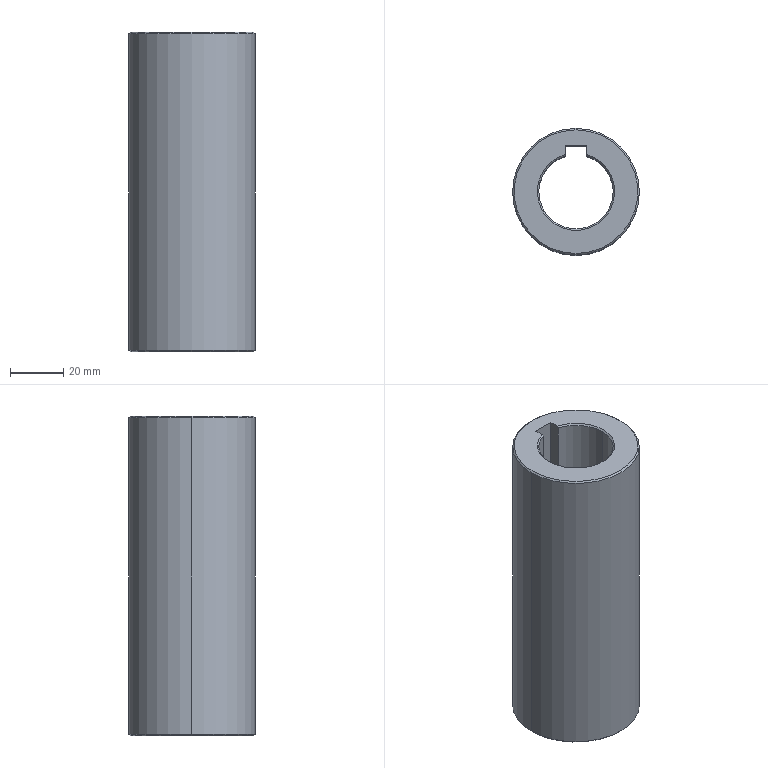Part | SolidWorks | features BaseBody 1 | 1 solid | 32 faces | box 47.6 x 47.6 x 120 mm | volume 130851 mm3 | cone 16 | cylinder 11 | plane 5 | commonest cylinder face diameters 28 x6 31.3 x3 47.6 x2
STEP:
#1=CARTESIAN_POINT('',(0.,23.8,-59.44));
#2=VERTEX_POINT('',#1);
#3=CARTESIAN_POINT('',(-23.8,0.,-59.44));
#4=VERTEX_POINT('',#3);
#5=CARTESIAN_POINT('',(0.,0.,-59.44));
#6=DIRECTION('',(0.,0.,1.));
#7=DIRECTION('',(1.,0.,0.));
#8=AXIS2_PLACEMENT_3D('',#5,#6,#7);
#9=CIRCLE('',#8,23.8);
#10=EDGE_CURVE('',#2,#4,#9,.T.);
#11=ORIENTED_EDGE('',*,*,#10,.T.);
#12=CARTESIAN_POINT('',(-23.8,0.,59.44));
#13=VERTEX_POINT('',#12);
#14=CARTESIAN_POINT('',(-23.8,0.,60.));
#15=DIRECTION('',(0.,0.,1.));
#16=VECTOR('',#15,1000.);
#17=LINE('',#14,#16);
#18=EDGE_CURVE('',#4,#13,#17,.T.);
#19=ORIENTED_EDGE('',*,*,#18,.T.);
#20=CARTESIAN_POINT('',(0.,23.8,59.44));
#21=VERTEX_POINT('',#20);
#22=CARTESIAN_POINT('',(0.,0.,59.44));
#23=DIRECTION('',(0.,0.,-1.));
#24=DIRECTION('',(1.,0.,0.));
#25=AXIS2_PLACEMENT_3D('',#22,#23,#24);
#26=CIRCLE('',#25,23.8);
#27=EDGE_CURVE('',#13,#21,#26,.T.);
#28=ORIENTED_EDGE('',*,*,#27,.T.);
#29=CARTESIAN_POINT('',(23.8,0.,59.44));
#30=VERTEX_POINT('',#29);
#31=CARTESIAN_POINT('',(0.,0.,59.44));
#32=DIRECTION('',(0.,0.,-1.));
#33=DIRECTION('',(1.,0.,0.));
#34=AXIS2_PLACEMENT_3D('',#31,#32,#33);
#35=CIRCLE('',#34,23.8);
#36=EDGE_CURVE('',#21,#30,#35,.T.);
#37=ORIENTED_EDGE('',*,*,#36,.T.);
#38=CARTESIAN_POINT('',(23.8,0.,-59.44));
#39=VERTEX_POINT('',#38);
#40=CARTESIAN_POINT('',(23.8,0.,60.));
#41=DIRECTION('',(0.,0.,1.));
#42=VECTOR('',#41,1000.);
#43=LINE('',#40,#42);
#44=EDGE_CURVE('',#39,#30,#43,.T.);
#45=ORIENTED_EDGE('',*,*,#44,.F.);
#46=CARTESIAN_POINT('',(0.,0.,-59.44));
#47=DIRECTION('',(0.,0.,1.));
#48=DIRECTION('',(1.,0.,0.));
#49=AXIS2_PLACEMENT_3D('',#46,#47,#48);
#50=CIRCLE('',#49,23.8);
#51=EDGE_CURVE('',#39,#2,#50,.T.);
#52=ORIENTED_EDGE('',*,*,#51,.T.);
#53=EDGE_LOOP('',(#11,#19,#28,#37,#45,#52));
#54=FACE_OUTER_BOUND('',#53,.T.);
#55=CARTESIAN_POINT('',(0.,0.,60.));
#56=DIRECTION('',(0.,0.,1.));
#57=DIRECTION('',(1.,0.,0.));
#58=AXIS2_PLACEMENT_3D('',#55,#56,#57);
#59=CYLINDRICAL_SURFACE('',#58,23.8);
#60=ADVANCED_FACE('',(#54),#59,.T.);
#61=CARTESIAN_POINT('',(0.,23.24,60.));
#62=VERTEX_POINT('',#61);
#63=CARTESIAN_POINT('',(0.,-23.24,60.));
#64=VERTEX_POINT('',#63);
#65=CARTESIAN_POINT('',(0.,0.,60.));
#66=DIRECTION('',(0.,0.,-1.));
#67=DIRECTION('',(0.,1.,0.));
#68=AXIS2_PLACEMENT_3D('',#65,#66,#67);
#69=CIRCLE('',#68,23.24);
#70=EDGE_CURVE('',#62,#64,#69,.T.);
#71=ORIENTED_EDGE('',*,*,#70,.T.);
#72=CARTESIAN_POINT('',(0.,-23.8,59.44));
#73=VERTEX_POINT('',#72);
#74=CARTESIAN_POINT('',(0.,-23.8,59.44));
#75=DIRECTION('',(0.,-0.7071,-0.7071));
#76=VECTOR('',#75,1000.);
#77=LINE('',#74,#76);
#78=EDGE_CURVE('',#64,#73,#77,.T.);
#79=ORIENTED_EDGE('',*,*,#78,.T.);
#80=CARTESIAN_POINT('',(0.,0.,59.44));
#81=DIRECTION('',(0.,0.,-1.));
#82=DIRECTION('',(1.,0.,0.));
#83=AXIS2_PLACEMENT_3D('',#80,#81,#82);
#84=CIRCLE('',#83,23.8);
#85=EDGE_CURVE('',#30,#73,#84,.T.);
#86=ORIENTED_EDGE('',*,*,#85,.F.);
#87=ORIENTED_EDGE('',*,*,#36,.F.);
#88=CARTESIAN_POINT('',(0.,23.8,59.44));
#89=DIRECTION('',(0.,0.7071,-0.7071));
#90=VECTOR('',#89,1000.);
#91=LINE('',#88,#90);
#92=EDGE_CURVE('',#62,#21,#91,.T.);
#93=ORIENTED_EDGE('',*,*,#92,.F.);
#94=EDGE_LOOP('',(#71,#79,#86,#87,#93));
#95=FACE_OUTER_BOUND('',#94,.T.);
#96=CARTESIAN_POINT('',(0.,0.,59.44));
#97=DIRECTION('',(0.,0.,-1.));
#98=DIRECTION('',(0.,1.,0.));
#99=AXIS2_PLACEMENT_3D('',#96,#97,#98);
#100=CONICAL_SURFACE('',#99,23.8,0.7854);
#101=ADVANCED_FACE('',(#95),#100,.T.);
#102=CARTESIAN_POINT('',(0.,-23.24,-60.));
#103=VERTEX_POINT('',#102);
#104=CARTESIAN_POINT('',(0.,23.24,-60.));
#105=VERTEX_POINT('',#104);
#106=CARTESIAN_POINT('',(0.,0.,-60.));
#107=DIRECTION('',(0.,0.,1.));
#108=DIRECTION('',(0.,-1.,0.));
#109=AXIS2_PLACEMENT_3D('',#106,#107,#108);
#110=CIRCLE('',#109,23.24);
#111=EDGE_CURVE('',#103,#105,#110,.T.);
#112=ORIENTED_EDGE('',*,*,#111,.T.);
#113=CARTESIAN_POINT('',(0.,23.8,-59.44));
#114=DIRECTION('',(0.,0.7071,0.7071));
#115=VECTOR('',#114,1000.);
#116=LINE('',#113,#115);
#117=EDGE_CURVE('',#105,#2,#116,.T.);
#118=ORIENTED_EDGE('',*,*,#117,.T.);
#119=ORIENTED_EDGE('',*,*,#51,.F.);
#120=CARTESIAN_POINT('',(0.,-23.8,-59.44));
#121=VERTEX_POINT('',#120);
#122=CARTESIAN_POINT('',(0.,0.,-59.44));
#123=DIRECTION('',(0.,0.,1.));
#124=DIRECTION('',(1.,0.,0.));
#125=AXIS2_PLACEMENT_3D('',#122,#123,#124);
#126=CIRCLE('',#125,23.8);
#127=EDGE_CURVE('',#121,#39,#126,.T.);
#128=ORIENTED_EDGE('',*,*,#127,.F.);
#129=CARTESIAN_POINT('',(0.,-23.8,-59.44));
#130=DIRECTION('',(0.,-0.7071,0.7071));
#131=VECTOR('',#130,1000.);
#132=LINE('',#129,#131);
#133=EDGE_CURVE('',#103,#121,#132,.T.);
#134=ORIENTED_EDGE('',*,*,#133,.F.);
#135=EDGE_LOOP('',(#112,#118,#119,#128,#134));
#136=FACE_OUTER_BOUND('',#135,.T.);
#137=CARTESIAN_POINT('',(0.,0.,-59.44));
#138=DIRECTION('',(0.,0.,1.));
#139=DIRECTION('',(0.,-1.,0.));
#140=AXIS2_PLACEMENT_3D('',#137,#138,#139);
#141=CONICAL_SURFACE('',#140,23.8,0.7854);
#142=ADVANCED_FACE('',(#136),#141,.T.);
#143=CARTESIAN_POINT('',(-14.,0.,59.44));
#144=VERTEX_POINT('',#143);
#145=CARTESIAN_POINT('',(14.,0.,59.44));
#146=VERTEX_POINT('',#145);
#147=CARTESIAN_POINT('',(0.,0.,59.44));
#148=DIRECTION('',(0.,0.,1.));
#149=DIRECTION('',(1.,0.,0.));
#150=AXIS2_PLACEMENT_3D('',#147,#148,#149);
#151=CIRCLE('',#150,14.);
#152=EDGE_CURVE('',#144,#146,#151,.T.);
#153=ORIENTED_EDGE('',*,*,#152,.F.);
#154=CARTESIAN_POINT('',(-14.56,0.,60.));
#155=VERTEX_POINT('',#154);
#156=CARTESIAN_POINT('',(-14.56,0.,60.));
#157=DIRECTION('',(-0.7071,0.,0.7071));
#158=VECTOR('',#157,1000.);
#159=LINE('',#156,#158);
#160=EDGE_CURVE('',#144,#155,#159,.T.);
#161=ORIENTED_EDGE('',*,*,#160,.T.);
#162=CARTESIAN_POINT('',(14.56,0.,60.));
#163=VERTEX_POINT('',#162);
#164=CARTESIAN_POINT('',(0.,0.,60.));
#165=DIRECTION('',(0.,0.,1.));
#166=DIRECTION('',(1.,0.,0.));
#167=AXIS2_PLACEMENT_3D('',#164,#165,#166);
#168=CIRCLE('',#167,14.56);
#169=EDGE_CURVE('',#155,#163,#168,.T.);
#170=ORIENTED_EDGE('',*,*,#169,.T.);
#171=CARTESIAN_POINT('',(14.56,0.,60.));
#172=DIRECTION('',(0.7071,0.,0.7071));
#173=VECTOR('',#172,1000.);
#174=LINE('',#171,#173);
#175=EDGE_CURVE('',#146,#163,#174,.T.);
#176=ORIENTED_EDGE('',*,*,#175,.F.);
#177=EDGE_LOOP('',(#153,#161,#170,#176));
#178=FACE_OUTER_BOUND('',#177,.T.);
#179=CARTESIAN_POINT('',(0.,0.,60.));
#180=DIRECTION('',(0.,0.,1.));
#181=DIRECTION('',(1.,0.,0.));
#182=AXIS2_PLACEMENT_3D('',#179,#180,#181);
#183=CONICAL_SURFACE('',#182,14.56,0.7854);
#184=ADVANCED_FACE('',(#178),#183,.F.);
#185=CARTESIAN_POINT('',(4.,13.416,59.44));
#186=VERTEX_POINT('',#185);
#187=CARTESIAN_POINT('',(0.,0.,59.44));
#188=DIRECTION('',(0.,0.,1.));
#189=DIRECTION('',(1.,0.,0.));
#190=AXIS2_PLACEMENT_3D('',#187,#188,#189);
#191=CIRCLE('',#190,14.);
#192=EDGE_CURVE('',#146,#186,#191,.T.);
#193=ORIENTED_EDGE('',*,*,#192,.F.);
#194=ORIENTED_EDGE('',*,*,#175,.T.);
#195=CARTESIAN_POINT('',(4.,14.,60.));
#196=VERTEX_POINT('',#195);
#197=CARTESIAN_POINT('',(0.,0.,60.));
#198=DIRECTION('',(0.,0.,1.));
#199=DIRECTION('',(1.,0.,0.));
#200=AXIS2_PLACEMENT_3D('',#197,#198,#199);
#201=CIRCLE('',#200,14.56);
#202=EDGE_CURVE('',#163,#196,#201,.T.);
#203=ORIENTED_EDGE('',*,*,#202,.T.);
#204=CARTESIAN_POINT('',(4.,14.,60.));
#205=CARTESIAN_POINT('',(4.,13.805,59.813));
#206=CARTESIAN_POINT('',(4.,13.611,59.627));
#207=CARTESIAN_POINT('',(4.,13.416,59.44));
#208=B_SPLINE_CURVE_WITH_KNOTS('',3,(#204,#205,#206,#207),.UNSPECIFIED.,.F.,.F.,(4,4),(0.,0.0008086),.UNSPECIFIED.);
#209=EDGE_CURVE('',#196,#186,#208,.T.);
#210=ORIENTED_EDGE('',*,*,#209,.T.);
#211=EDGE_LOOP('',(#193,#194,#203,#210));
#212=FACE_OUTER_BOUND('',#211,.T.);
#213=CARTESIAN_POINT('',(0.,0.,60.));
#214=DIRECTION('',(0.,0.,1.));
#215=DIRECTION('',(1.,0.,0.));
#216=AXIS2_PLACEMENT_3D('',#213,#214,#215);
#217=CONICAL_SURFACE('',#216,14.56,0.7854);
#218=ADVANCED_FACE('',(#212),#217,.F.);
#219=CARTESIAN_POINT('',(14.,0.,-59.44));
#220=VERTEX_POINT('',#219);
#221=CARTESIAN_POINT('',(-14.,0.,-59.44));
#222=VERTEX_POINT('',#221);
#223=CARTESIAN_POINT('',(0.,0.,-59.44));
#224=DIRECTION('',(0.,0.,-1.));
#225=DIRECTION('',(-1.,0.,0.));
#226=AXIS2_PLACEMENT_3D('',#223,#224,#225);
#227=CIRCLE('',#226,14.);
#228=EDGE_CURVE('',#220,#222,#227,.T.);
#229=ORIENTED_EDGE('',*,*,#228,.F.);
#230=CARTESIAN_POINT('',(14.56,0.,-60.));
#231=VERTEX_POINT('',#230);
#232=CARTESIAN_POINT('',(14.56,0.,-60.));
#233=DIRECTION('',(0.7071,0.,-0.7071));
#234=VECTOR('',#233,1000.);
#235=LINE('',#232,#234);
#236=EDGE_CURVE('',#220,#231,#235,.T.);
#237=ORIENTED_EDGE('',*,*,#236,.T.);
#238=CARTESIAN_POINT('',(-14.56,0.,-60.));
#239=VERTEX_POINT('',#238);
#240=CARTESIAN_POINT('',(0.,0.,-60.));
#241=DIRECTION('',(0.,0.,-1.));
#242=DIRECTION('',(-1.,0.,0.));
#243=AXIS2_PLACEMENT_3D('',#240,#241,#242);
#244=CIRCLE('',#243,14.56);
#245=EDGE_CURVE('',#231,#239,#244,.T.);
#246=ORIENTED_EDGE('',*,*,#245,.T.);
#247=CARTESIAN_POINT('',(-14.56,0.,-60.));
#248=DIRECTION('',(-0.7071,0.,-0.7071));
#249=VECTOR('',#248,1000.);
#250=LINE('',#247,#249);
#251=EDGE_CURVE('',#222,#239,#250,.T.);
#252=ORIENTED_EDGE('',*,*,#251,.F.);
#253=EDGE_LOOP('',(#229,#237,#246,#252));
#254=FACE_OUTER_BOUND('',#253,.T.);
#255=CARTESIAN_POINT('',(0.,0.,-60.));
#256=DIRECTION('',(0.,0.,-1.));
#257=DIRECTION('',(-1.,0.,0.));
#258=AXIS2_PLACEMENT_3D('',#255,#256,#257);
#259=CONICAL_SURFACE('',#258,14.56,0.7854);
#260=ADVANCED_FACE('',(#254),#259,.F.);
#261=CARTESIAN_POINT('',(-4.,13.416,-59.44));
#262=VERTEX_POINT('',#261);
#263=CARTESIAN_POINT('',(0.,0.,-59.44));
#264=DIRECTION('',(0.,0.,-1.));
#265=DIRECTION('',(-1.,0.,0.));
#266=AXIS2_PLACEMENT_3D('',#263,#264,#265);
#267=CIRCLE('',#266,14.);
#268=EDGE_CURVE('',#222,#262,#267,.T.);
#269=ORIENTED_EDGE('',*,*,#268,.F.);
#270=ORIENTED_EDGE('',*,*,#251,.T.);
#271=CARTESIAN_POINT('',(-4.,14.,-60.));
#272=VERTEX_POINT('',#271);
#273=CARTESIAN_POINT('',(0.,0.,-60.));
#274=DIRECTION('',(0.,0.,-1.));
#275=DIRECTION('',(-1.,0.,0.));
#276=AXIS2_PLACEMENT_3D('',#273,#274,#275);
#277=CIRCLE('',#276,14.56);
#278=EDGE_CURVE('',#239,#272,#277,.T.);
#279=ORIENTED_EDGE('',*,*,#278,.T.);
#280=CARTESIAN_POINT('',(-4.,14.,-60.));
#281=CARTESIAN_POINT('',(-4.,13.805,-59.813));
#282=CARTESIAN_POINT('',(-4.,13.611,-59.627));
#283=CARTESIAN_POINT('',(-4.,13.416,-59.44));
#284=B_SPLINE_CURVE_WITH_KNOTS('',3,(#280,#281,#282,#283),.UNSPECIFIED.,.F.,.F.,(4,4),(0.,0.0008086),.UNSPECIFIED.);
#285=EDGE_CURVE('',#272,#262,#284,.T.);
#286=ORIENTED_EDGE('',*,*,#285,.T.);
#287=EDGE_LOOP('',(#269,#270,#279,#286));
#288=FACE_OUTER_BOUND('',#287,.T.);
#289=CARTESIAN_POINT('',(0.,0.,-60.));
#290=DIRECTION('',(0.,0.,-1.));
#291=DIRECTION('',(-1.,0.,0.));
#292=AXIS2_PLACEMENT_3D('',#289,#290,#291);
#293=CONICAL_SURFACE('',#292,14.56,0.7854);
#294=ADVANCED_FACE('',(#288),#293,.F.);
#295=CARTESIAN_POINT('',(-14.,0.,20.));
#296=VERTEX_POINT('',#295);
#297=CARTESIAN_POINT('',(14.,0.,20.));
#298=VERTEX_POINT('',#297);
#299=CARTESIAN_POINT('',(0.,0.,20.));
#300=DIRECTION('',(0.,0.,1.));
#301=DIRECTION('',(1.,0.,0.));
#302=AXIS2_PLACEMENT_3D('',#299,#300,#301);
#303=CIRCLE('',#302,14.);
#304=EDGE_CURVE('',#296,#298,#303,.T.);
#305=ORIENTED_EDGE('',*,*,#304,.F.);
#306=CARTESIAN_POINT('',(-14.,0.,60.));
#307=DIRECTION('',(0.,0.,1.));
#308=VECTOR('',#307,1000.);
#309=LINE('',#306,#308);
#310=EDGE_CURVE('',#296,#144,#309,.T.);
#311=ORIENTED_EDGE('',*,*,#310,.T.);
#312=ORIENTED_EDGE('',*,*,#152,.T.);
#313=CARTESIAN_POINT('',(14.,0.,60.));
#314=DIRECTION('',(0.,0.,1.));
#315=VECTOR('',#314,1000.);
#316=LINE('',#313,#315);
#317=EDGE_CURVE('',#298,#146,#316,.T.);
#318=ORIENTED_EDGE('',*,*,#317,.F.);
#319=EDGE_LOOP('',(#305,#311,#312,#318));
#320=FACE_OUTER_BOUND('',#319,.T.);
#321=CARTESIAN_POINT('',(0.,0.,60.));
#322=DIRECTION('',(0.,0.,1.));
#323=DIRECTION('',(1.,0.,0.));
#324=AXIS2_PLACEMENT_3D('',#321,#322,#323);
#325=CYLINDRICAL_SURFACE('',#324,14.);
#326=ADVANCED_FACE('',(#320),#325,.F.);
#327=CARTESIAN_POINT('',(4.,13.416,20.));
#328=VERTEX_POINT('',#327);
#329=CARTESIAN_POINT('',(0.,0.,20.));
#330=DIRECTION('',(0.,0.,1.));
#331=DIRECTION('',(1.,0.,0.));
#332=AXIS2_PLACEMENT_3D('',#329,#330,#331);
#333=CIRCLE('',#332,14.);
#334=EDGE_CURVE('',#298,#328,#333,.T.);
#335=ORIENTED_EDGE('',*,*,#334,.F.);
#336=ORIENTED_EDGE('',*,*,#317,.T.);
#337=ORIENTED_EDGE('',*,*,#192,.T.);
#338=CARTESIAN_POINT('',(4.,13.416,-60.));
#339=DIRECTION('',(0.,0.,-1.));
#340=VECTOR('',#339,1000.);
#341=LINE('',#338,#340);
#342=EDGE_CURVE('',#186,#328,#341,.T.);
#343=ORIENTED_EDGE('',*,*,#342,.T.);
#344=EDGE_LOOP('',(#335,#336,#337,#343));
#345=FACE_OUTER_BOUND('',#344,.T.);
#346=CARTESIAN_POINT('',(0.,0.,60.));
#347=DIRECTION('',(0.,0.,1.));
#348=DIRECTION('',(1.,0.,0.));
#349=AXIS2_PLACEMENT_3D('',#346,#347,#348);
#350=CYLINDRICAL_SURFACE('',#349,14.);
#351=ADVANCED_FACE('',(#345),#350,.F.);
#352=CARTESIAN_POINT('',(-15.65,0.,-18.35));
#353=VERTEX_POINT('',#352);
#354=CARTESIAN_POINT('',(15.65,0.,-18.35));
#355=VERTEX_POINT('',#354);
#356=CARTESIAN_POINT('',(0.,0.,-18.35));
#357=DIRECTION('',(0.,0.,1.));
#358=DIRECTION('',(1.,0.,0.));
#359=AXIS2_PLACEMENT_3D('',#356,#357,#358);
#360=CIRCLE('',#359,15.65);
#361=EDGE_CURVE('',#353,#355,#360,.T.);
#362=ORIENTED_EDGE('',*,*,#361,.F.);
#363=CARTESIAN_POINT('',(-15.65,0.,18.35));
#364=VERTEX_POINT('',#363);
#365=CARTESIAN_POINT('',(-15.65,0.,60.));
#366=DIRECTION('',(0.,0.,1.));
#367=VECTOR('',#366,1000.);
#368=LINE('',#365,#367);
#369=EDGE_CURVE('',#353,#364,#368,.T.);
#370=ORIENTED_EDGE('',*,*,#369,.T.);
#371=CARTESIAN_POINT('',(15.65,0.,18.35));
#372=VERTEX_POINT('',#371);
#373=CARTESIAN_POINT('',(0.,0.,18.35));
#374=DIRECTION('',(0.,0.,-1.));
#375=DIRECTION('',(1.,0.,0.));
#376=AXIS2_PLACEMENT_3D('',#373,#374,#375);
#377=CIRCLE('',#376,15.65);
#378=EDGE_CURVE('',#372,#364,#377,.T.);
#379=ORIENTED_EDGE('',*,*,#378,.F.);
#380=CARTESIAN_POINT('',(15.65,0.,60.));
#381=DIRECTION('',(0.,0.,1.));
#382=VECTOR('',#381,1000.);
#383=LINE('',#380,#382);
#384=EDGE_CURVE('',#355,#372,#383,.T.);
#385=ORIENTED_EDGE('',*,*,#384,.F.);
#386=EDGE_LOOP('',(#362,#370,#379,#385));
#387=FACE_OUTER_BOUND('',#386,.T.);
#388=CARTESIAN_POINT('',(0.,0.,60.));
#389=DIRECTION('',(0.,0.,1.));
#390=DIRECTION('',(1.,0.,0.));
#391=AXIS2_PLACEMENT_3D('',#388,#389,#390);
#392=CYLINDRICAL_SURFACE('',#391,15.65);
#393=ADVANCED_FACE('',(#387),#392,.F.);
#394=CARTESIAN_POINT('',(4.,15.13,-18.35));
#395=VERTEX_POINT('',#394);
#396=CARTESIAN_POINT('',(0.,0.,-18.35));
#397=DIRECTION('',(0.,0.,1.));
#398=DIRECTION('',(1.,0.,0.));
#399=AXIS2_PLACEMENT_3D('',#396,#397,#398);
#400=CIRCLE('',#399,15.65);
#401=EDGE_CURVE('',#355,#395,#400,.T.);
#402=ORIENTED_EDGE('',*,*,#401,.F.);
#403=ORIENTED_EDGE('',*,*,#384,.T.);
#404=CARTESIAN_POINT('',(4.,15.13,18.35));
#405=VERTEX_POINT('',#404);
#406=CARTESIAN_POINT('',(0.,0.,18.35));
#407=DIRECTION('',(0.,0.,-1.));
#408=DIRECTION('',(1.,0.,0.));
#409=AXIS2_PLACEMENT_3D('',#406,#407,#408);
#410=CIRCLE('',#409,15.65);
#411=EDGE_CURVE('',#405,#372,#410,.T.);
#412=ORIENTED_EDGE('',*,*,#411,.F.);
#413=CARTESIAN_POINT('',(4.,15.13,-60.));
#414=DIRECTION('',(0.,0.,-1.));
#415=VECTOR('',#414,1000.);
#416=LINE('',#413,#415);
#417=EDGE_CURVE('',#405,#395,#416,.T.);
#418=ORIENTED_EDGE('',*,*,#417,.T.);
#419=EDGE_LOOP('',(#402,#403,#412,#418));
#420=FACE_OUTER_BOUND('',#419,.T.);
#421=CARTESIAN_POINT('',(0.,0.,60.));
#422=DIRECTION('',(0.,0.,1.));
#423=DIRECTION('',(1.,0.,0.));
#424=AXIS2_PLACEMENT_3D('',#421,#422,#423);
#425=CYLINDRICAL_SURFACE('',#424,15.65);
#426=ADVANCED_FACE('',(#420),#425,.F.);
#427=CARTESIAN_POINT('',(-14.,0.,-20.));
#428=VERTEX_POINT('',#427);
#429=CARTESIAN_POINT('',(14.,0.,-20.));
#430=VERTEX_POINT('',#429);
#431=CARTESIAN_POINT('',(0.,0.,-20.));
#432=DIRECTION('',(0.,0.,1.));
#433=DIRECTION('',(1.,0.,0.));
#434=AXIS2_PLACEMENT_3D('',#431,#432,#433);
#435=CIRCLE('',#434,14.);
#436=EDGE_CURVE('',#428,#430,#435,.T.);
#437=ORIENTED_EDGE('',*,*,#436,.F.);
#438=CARTESIAN_POINT('',(-15.65,0.,-18.35));
#439=DIRECTION('',(-0.7071,0.,0.7071));
#440=VECTOR('',#439,1000.);
#441=LINE('',#438,#440);
#442=EDGE_CURVE('',#428,#353,#441,.T.);
#443=ORIENTED_EDGE('',*,*,#442,.T.);
#444=ORIENTED_EDGE('',*,*,#361,.T.);
#445=CARTESIAN_POINT('',(15.65,0.,-18.35));
#446=DIRECTION('',(0.7071,0.,0.7071));
#447=VECTOR('',#446,1000.);
#448=LINE('',#445,#447);
#449=EDGE_CURVE('',#430,#355,#448,.T.);
#450=ORIENTED_EDGE('',*,*,#449,.F.);
#451=EDGE_LOOP('',(#437,#443,#444,#450));
#452=FACE_OUTER_BOUND('',#451,.T.);
#453=CARTESIAN_POINT('',(0.,0.,-18.35));
#454=DIRECTION('',(0.,0.,1.));
#455=DIRECTION('',(1.,0.,0.));
#456=AXIS2_PLACEMENT_3D('',#453,#454,#455);
#457=CONICAL_SURFACE('',#456,15.65,0.7854);
#458=ADVANCED_FACE('',(#452),#457,.F.);
#459=CARTESIAN_POINT('',(4.,13.416,-20.));
#460=VERTEX_POINT('',#459);
#461=CARTESIAN_POINT('',(0.,0.,-20.));
#462=DIRECTION('',(0.,0.,1.));
#463=DIRECTION('',(1.,0.,0.));
#464=AXIS2_PLACEMENT_3D('',#461,#462,#463);
#465=CIRCLE('',#464,14.);
#466=EDGE_CURVE('',#430,#460,#465,.T.);
#467=ORIENTED_EDGE('',*,*,#466,.F.);
#468=ORIENTED_EDGE('',*,*,#449,.T.);
#469=ORIENTED_EDGE('',*,*,#401,.T.);
#470=CARTESIAN_POINT('',(4.,15.13,-18.35));
#471=CARTESIAN_POINT('',(4.,14.56,-18.901));
#472=CARTESIAN_POINT('',(4.,13.989,-19.451));
#473=CARTESIAN_POINT('',(4.,13.416,-20.));
#474=B_SPLINE_CURVE_WITH_KNOTS('',3,(#470,#471,#472,#473),.UNSPECIFIED.,.F.,.F.,(4,4),(0.,0.002379),.UNSPECIFIED.);
#475=EDGE_CURVE('',#395,#460,#474,.T.);
#476=ORIENTED_EDGE('',*,*,#475,.T.);
#477=EDGE_LOOP('',(#467,#468,#469,#476));
#478=FACE_OUTER_BOUND('',#477,.T.);
#479=CARTESIAN_POINT('',(0.,0.,-18.35));
#480=DIRECTION('',(0.,0.,1.));
#481=DIRECTION('',(1.,0.,0.));
#482=AXIS2_PLACEMENT_3D('',#479,#480,#481);
#483=CONICAL_SURFACE('',#482,15.65,0.7854);
#484=ADVANCED_FACE('',(#478),#483,.F.);
#485=ORIENTED_EDGE('',*,*,#228,.T.);
#486=CARTESIAN_POINT('',(-14.,0.,60.));
#487=DIRECTION('',(0.,0.,1.));
#488=VECTOR('',#487,1000.);
#489=LINE('',#486,#488);
#490=EDGE_CURVE('',#222,#428,#489,.T.);
#491=ORIENTED_EDGE('',*,*,#490,.T.);
#492=ORIENTED_EDGE('',*,*,#436,.T.);
#493=CARTESIAN_POINT('',(14.,0.,60.));
#494=DIRECTION('',(0.,0.,1.));
#495=VECTOR('',#494,1000.);
#496=LINE('',#493,#495);
#497=EDGE_CURVE('',#220,#430,#496,.T.);
#498=ORIENTED_EDGE('',*,*,#497,.F.);
#499=EDGE_LOOP('',(#485,#491,#492,#498));
#500=FACE_OUTER_BOUND('',#499,.T.);
#501=CARTESIAN_POINT('',(0.,0.,60.));
#502=DIRECTION('',(0.,0.,1.));
#503=DIRECTION('',(1.,0.,0.));
#504=AXIS2_PLACEMENT_3D('',#501,#502,#503);
#505=CYLINDRICAL_SURFACE('',#504,14.);
#506=ADVANCED_FACE('',(#500),#505,.F.);
#507=CARTESIAN_POINT('',(4.,13.416,-59.44));
#508=VERTEX_POINT('',#507);
#509=CARTESIAN_POINT('',(0.,0.,-59.44));
#510=DIRECTION('',(0.,0.,-1.));
#511=DIRECTION('',(-1.,0.,0.));
#512=AXIS2_PLACEMENT_3D('',#509,#510,#511);
#513=CIRCLE('',#512,14.);
#514=EDGE_CURVE('',#508,#220,#513,.T.);
#515=ORIENTED_EDGE('',*,*,#514,.T.);
#516=ORIENTED_EDGE('',*,*,#497,.T.);
#517=ORIENTED_EDGE('',*,*,#466,.T.);
#518=CARTESIAN_POINT('',(4.,13.416,-60.));
#519=DIRECTION('',(0.,0.,-1.));
#520=VECTOR('',#519,1000.);
#521=LINE('',#518,#520);
#522=EDGE_CURVE('',#460,#508,#521,.T.);
#523=ORIENTED_EDGE('',*,*,#522,.T.);
#524=EDGE_LOOP('',(#515,#516,#517,#523));
#525=FACE_OUTER_BOUND('',#524,.T.);
#526=CARTESIAN_POINT('',(0.,0.,60.));
#527=DIRECTION('',(0.,0.,1.));
#528=DIRECTION('',(1.,0.,0.));
#529=AXIS2_PLACEMENT_3D('',#526,#527,#528);
#530=CYLINDRICAL_SURFACE('',#529,14.);
#531=ADVANCED_FACE('',(#525),#530,.F.);
#532=ORIENTED_EDGE('',*,*,#304,.T.);
#533=CARTESIAN_POINT('',(15.65,0.,18.35));
#534=DIRECTION('',(0.7071,0.,-0.7071));
#535=VECTOR('',#534,1000.);
#536=LINE('',#533,#535);
#537=EDGE_CURVE('',#298,#372,#536,.T.);
#538=ORIENTED_EDGE('',*,*,#537,.T.);
#539=ORIENTED_EDGE('',*,*,#378,.T.);
#540=CARTESIAN_POINT('',(-15.65,0.,18.35));
#541=DIRECTION('',(-0.7071,0.,-0.7071));
#542=VECTOR('',#541,1000.);
#543=LINE('',#540,#542);
#544=EDGE_CURVE('',#296,#364,#543,.T.);
#545=ORIENTED_EDGE('',*,*,#544,.F.);
#546=EDGE_LOOP('',(#532,#538,#539,#545));
#547=FACE_OUTER_BOUND('',#546,.T.);
#548=CARTESIAN_POINT('',(0.,0.,18.35));
#549=DIRECTION('',(0.,0.,-1.));
#550=DIRECTION('',(-1.,0.,0.));
#551=AXIS2_PLACEMENT_3D('',#548,#549,#550);
#552=CONICAL_SURFACE('',#551,15.65,0.7854);
#553=ADVANCED_FACE('',(#547),#552,.F.);
#554=CARTESIAN_POINT('',(-4.,13.416,20.));
#555=VERTEX_POINT('',#554);
#556=CARTESIAN_POINT('',(0.,0.,20.));
#557=DIRECTION('',(0.,0.,1.));
#558=DIRECTION('',(1.,0.,0.));
#559=AXIS2_PLACEMENT_3D('',#556,#557,#558);
#560=CIRCLE('',#559,14.);
#561=EDGE_CURVE('',#555,#296,#560,.T.);
#562=ORIENTED_EDGE('',*,*,#561,.T.);
#563=ORIENTED_EDGE('',*,*,#544,.T.);
#564=CARTESIAN_POINT('',(-4.,15.13,18.35));
#565=VERTEX_POINT('',#564);
#566=CARTESIAN_POINT('',(0.,0.,18.35));
#567=DIRECTION('',(0.,0.,-1.));
#568=DIRECTION('',(1.,0.,0.));
#569=AXIS2_PLACEMENT_3D('',#566,#567,#568);
#570=CIRCLE('',#569,15.65);
#571=EDGE_CURVE('',#364,#565,#570,.T.);
#572=ORIENTED_EDGE('',*,*,#571,.T.);
#573=CARTESIAN_POINT('',(-4.,15.13,18.35));
#574=CARTESIAN_POINT('',(-4.,14.56,18.901));
#575=CARTESIAN_POINT('',(-4.,13.989,19.451));
#576=CARTESIAN_POINT('',(-4.,13.416,20.));
#577=B_SPLINE_CURVE_WITH_KNOTS('',3,(#573,#574,#575,#576),.UNSPECIFIED.,.F.,.F.,(4,4),(0.,0.002379),.UNSPECIFIED.);
#578=EDGE_CURVE('',#565,#555,#577,.T.);
#579=ORIENTED_EDGE('',*,*,#578,.T.);
#580=EDGE_LOOP('',(#562,#563,#572,#579));
#581=FACE_OUTER_BOUND('',#580,.T.);
#582=CARTESIAN_POINT('',(0.,0.,18.35));
#583=DIRECTION('',(0.,0.,-1.));
#584=DIRECTION('',(-1.,0.,0.));
#585=AXIS2_PLACEMENT_3D('',#582,#583,#584);
#586=CONICAL_SURFACE('',#585,15.65,0.7854);
#587=ADVANCED_FACE('',(#581),#586,.F.);
#588=ORIENTED_EDGE('',*,*,#18,.F.);
#589=CARTESIAN_POINT('',(0.,0.,-59.44));
#590=DIRECTION('',(0.,0.,1.));
#591=DIRECTION('',(1.,0.,0.));
#592=AXIS2_PLACEMENT_3D('',#589,#590,#591);
#593=CIRCLE('',#592,23.8);
#594=EDGE_CURVE('',#4,#121,#593,.T.);
#595=ORIENTED_EDGE('',*,*,#594,.T.);
#596=ORIENTED_EDGE('',*,*,#127,.T.);
#597=ORIENTED_EDGE('',*,*,#44,.T.);
#598=ORIENTED_EDGE('',*,*,#85,.T.);
#599=CARTESIAN_POINT('',(0.,0.,59.44));
#600=DIRECTION('',(0.,0.,-1.));
#601=DIRECTION('',(1.,0.,0.));
#602=AXIS2_PLACEMENT_3D('',#599,#600,#601);
#603=CIRCLE('',#602,23.8);
#604=EDGE_CURVE('',#73,#13,#603,.T.);
#605=ORIENTED_EDGE('',*,*,#604,.T.);
#606=EDGE_LOOP('',(#588,#595,#596,#597,#598,#605));
#607=FACE_OUTER_BOUND('',#606,.T.);
#608=CARTESIAN_POINT('',(0.,0.,60.));
#609=DIRECTION('',(0.,0.,1.));
#610=DIRECTION('',(1.,0.,0.));
#611=AXIS2_PLACEMENT_3D('',#608,#609,#610);
#612=CYLINDRICAL_SURFACE('',#611,23.8);
#613=ADVANCED_FACE('',(#607),#612,.T.);
#614=ORIENTED_EDGE('',*,*,#78,.F.);
#615=CARTESIAN_POINT('',(0.,0.,60.));
#616=DIRECTION('',(0.,0.,-1.));
#617=DIRECTION('',(0.,1.,0.));
#618=AXIS2_PLACEMENT_3D('',#615,#616,#617);
#619=CIRCLE('',#618,23.24);
#620=EDGE_CURVE('',#64,#62,#619,.T.);
#621=ORIENTED_EDGE('',*,*,#620,.T.);
#622=ORIENTED_EDGE('',*,*,#92,.T.);
#623=ORIENTED_EDGE('',*,*,#27,.F.);
#624=ORIENTED_EDGE('',*,*,#604,.F.);
#625=EDGE_LOOP('',(#614,#621,#622,#623,#624));
#626=FACE_OUTER_BOUND('',#625,.T.);
#627=CARTESIAN_POINT('',(0.,0.,59.44));
#628=DIRECTION('',(0.,0.,-1.));
#629=DIRECTION('',(0.,1.,0.));
#630=AXIS2_PLACEMENT_3D('',#627,#628,#629);
#631=CONICAL_SURFACE('',#630,23.8,0.7854);
#632=ADVANCED_FACE('',(#626),#631,.T.);
#633=ORIENTED_EDGE('',*,*,#117,.F.);
#634=CARTESIAN_POINT('',(0.,0.,-60.));
#635=DIRECTION('',(0.,0.,1.));
#636=DIRECTION('',(0.,-1.,0.));
#637=AXIS2_PLACEMENT_3D('',#634,#635,#636);
#638=CIRCLE('',#637,23.24);
#639=EDGE_CURVE('',#105,#103,#638,.T.);
#640=ORIENTED_EDGE('',*,*,#639,.T.);
#641=ORIENTED_EDGE('',*,*,#133,.T.);
#642=ORIENTED_EDGE('',*,*,#594,.F.);
#643=ORIENTED_EDGE('',*,*,#10,.F.);
#644=EDGE_LOOP('',(#633,#640,#641,#642,#643));
#645=FACE_OUTER_BOUND('',#644,.T.);
#646=CARTESIAN_POINT('',(0.,0.,-59.44));
#647=DIRECTION('',(0.,0.,1.));
#648=DIRECTION('',(0.,-1.,0.));
#649=AXIS2_PLACEMENT_3D('',#646,#647,#648);
#650=CONICAL_SURFACE('',#649,23.8,0.7854);
#651=ADVANCED_FACE('',(#645),#650,.T.);
#652=ORIENTED_EDGE('',*,*,#70,.F.);
#653=ORIENTED_EDGE('',*,*,#620,.F.);
#654=EDGE_LOOP('',(#652,#653));
#655=FACE_OUTER_BOUND('',#654,.T.);
#656=CARTESIAN_POINT('',(-4.,17.3,60.));
#657=VERTEX_POINT('',#656);
#658=CARTESIAN_POINT('',(-4.,14.,60.));
#659=VERTEX_POINT('',#658);
#660=CARTESIAN_POINT('',(-4.,14.56,60.));
#661=DIRECTION('',(0.,-1.,0.));
#662=VECTOR('',#661,1000.);
#663=LINE('',#660,#662);
#664=EDGE_CURVE('',#657,#659,#663,.T.);
#665=ORIENTED_EDGE('',*,*,#664,.F.);
#666=CARTESIAN_POINT('',(4.,17.3,60.));
#667=VERTEX_POINT('',#666);
#668=CARTESIAN_POINT('',(0.,17.3,60.));
#669=DIRECTION('',(-1.,0.,0.));
#670=VECTOR('',#669,1000.);
#671=LINE('',#668,#670);
#672=EDGE_CURVE('',#667,#657,#671,.T.);
#673=ORIENTED_EDGE('',*,*,#672,.F.);
#674=CARTESIAN_POINT('',(4.,14.56,60.));
#675=DIRECTION('',(0.,1.,0.));
#676=VECTOR('',#675,1000.);
#677=LINE('',#674,#676);
#678=EDGE_CURVE('',#196,#667,#677,.T.);
#679=ORIENTED_EDGE('',*,*,#678,.F.);
#680=ORIENTED_EDGE('',*,*,#202,.F.);
#681=ORIENTED_EDGE('',*,*,#169,.F.);
#682=CARTESIAN_POINT('',(0.,0.,60.));
#683=DIRECTION('',(0.,0.,1.));
#684=DIRECTION('',(1.,0.,0.));
#685=AXIS2_PLACEMENT_3D('',#682,#683,#684);
#686=CIRCLE('',#685,14.56);
#687=EDGE_CURVE('',#659,#155,#686,.T.);
#688=ORIENTED_EDGE('',*,*,#687,.F.);
#689=EDGE_LOOP('',(#665,#673,#679,#680,#681,#688));
#690=FACE_BOUND('',#689,.T.);
#691=CARTESIAN_POINT('',(0.,14.56,60.));
#692=DIRECTION('',(0.,0.,-1.));
#693=DIRECTION('',(-1.,0.,0.));
#694=AXIS2_PLACEMENT_3D('',#691,#692,#693);
#695=PLANE('',#694);
#696=ADVANCED_FACE('',(#655,#690),#695,.F.);
#697=CARTESIAN_POINT('',(-4.,17.3,-60.));
#698=VERTEX_POINT('',#697);
#699=CARTESIAN_POINT('',(-4.,23.24,-60.));
#700=DIRECTION('',(0.,1.,0.));
#701=VECTOR('',#700,1000.);
#702=LINE('',#699,#701);
#703=EDGE_CURVE('',#272,#698,#702,.T.);
#704=ORIENTED_EDGE('',*,*,#703,.F.);
#705=ORIENTED_EDGE('',*,*,#278,.F.);
#706=ORIENTED_EDGE('',*,*,#245,.F.);
#707=CARTESIAN_POINT('',(4.,14.,-60.));
#708=VERTEX_POINT('',#707);
#709=CARTESIAN_POINT('',(0.,0.,-60.));
#710=DIRECTION('',(0.,0.,-1.));
#711=DIRECTION('',(-1.,0.,0.));
#712=AXIS2_PLACEMENT_3D('',#709,#710,#711);
#713=CIRCLE('',#712,14.56);
#714=EDGE_CURVE('',#708,#231,#713,.T.);
#715=ORIENTED_EDGE('',*,*,#714,.F.);
#716=CARTESIAN_POINT('',(4.,17.3,-60.));
#717=VERTEX_POINT('',#716);
#718=CARTESIAN_POINT('',(4.,23.24,-60.));
#719=DIRECTION('',(0.,-1.,0.));
#720=VECTOR('',#719,1000.);
#721=LINE('',#718,#720);
#722=EDGE_CURVE('',#717,#708,#721,.T.);
#723=ORIENTED_EDGE('',*,*,#722,.F.);
#724=CARTESIAN_POINT('',(0.,17.3,-60.));
#725=DIRECTION('',(1.,0.,0.));
#726=VECTOR('',#725,1000.);
#727=LINE('',#724,#726);
#728=EDGE_CURVE('',#698,#717,#727,.T.);
#729=ORIENTED_EDGE('',*,*,#728,.F.);
#730=EDGE_LOOP('',(#704,#705,#706,#715,#723,#729));
#731=FACE_BOUND('',#730,.T.);
#732=ORIENTED_EDGE('',*,*,#111,.F.);
#733=ORIENTED_EDGE('',*,*,#639,.F.);
#734=EDGE_LOOP('',(#732,#733));
#735=FACE_OUTER_BOUND('',#734,.T.);
#736=CARTESIAN_POINT('',(0.,23.24,-60.));
#737=DIRECTION('',(0.,0.,1.));
#738=DIRECTION('',(1.,0.,0.));
#739=AXIS2_PLACEMENT_3D('',#736,#737,#738);
#740=PLANE('',#739);
#741=ADVANCED_FACE('',(#731,#735),#740,.F.);
#742=ORIENTED_EDGE('',*,*,#160,.F.);
#743=CARTESIAN_POINT('',(-4.,13.416,59.44));
#744=VERTEX_POINT('',#743);
#745=CARTESIAN_POINT('',(0.,0.,59.44));
#746=DIRECTION('',(0.,0.,1.));
#747=DIRECTION('',(1.,0.,0.));
#748=AXIS2_PLACEMENT_3D('',#745,#746,#747);
#749=CIRCLE('',#748,14.);
#750=EDGE_CURVE('',#744,#144,#749,.T.);
#751=ORIENTED_EDGE('',*,*,#750,.F.);
#752=CARTESIAN_POINT('',(-4.,14.,60.));
#753=CARTESIAN_POINT('',(-4.,13.805,59.813));
#754=CARTESIAN_POINT('',(-4.,13.611,59.627));
#755=CARTESIAN_POINT('',(-4.,13.416,59.44));
#756=B_SPLINE_CURVE_WITH_KNOTS('',3,(#752,#753,#754,#755),.UNSPECIFIED.,.F.,.F.,(4,4),(0.,0.0008086),.UNSPECIFIED.);
#757=EDGE_CURVE('',#659,#744,#756,.T.);
#758=ORIENTED_EDGE('',*,*,#757,.F.);
#759=ORIENTED_EDGE('',*,*,#687,.T.);
#760=EDGE_LOOP('',(#742,#751,#758,#759));
#761=FACE_OUTER_BOUND('',#760,.T.);
#762=CARTESIAN_POINT('',(0.,0.,60.));
#763=DIRECTION('',(0.,0.,1.));
#764=DIRECTION('',(1.,0.,0.));
#765=AXIS2_PLACEMENT_3D('',#762,#763,#764);
#766=CONICAL_SURFACE('',#765,14.56,0.7854);
#767=ADVANCED_FACE('',(#761),#766,.F.);
#768=CARTESIAN_POINT('',(-4.,13.416,-20.));
#769=VERTEX_POINT('',#768);
#770=CARTESIAN_POINT('',(-4.,15.13,-18.35));
#771=VERTEX_POINT('',#770);
#772=CARTESIAN_POINT('',(-4.,13.416,-20.));
#773=CARTESIAN_POINT('',(-4.,13.989,-19.451));
#774=CARTESIAN_POINT('',(-4.,14.56,-18.901));
#775=CARTESIAN_POINT('',(-4.,15.13,-18.35));
#776=B_SPLINE_CURVE_WITH_KNOTS('',3,(#772,#773,#774,#775),.UNSPECIFIED.,.F.,.F.,(4,4),(0.,0.002379),.UNSPECIFIED.);
#777=EDGE_CURVE('',#769,#771,#776,.T.);
#778=ORIENTED_EDGE('',*,*,#777,.F.);
#779=CARTESIAN_POINT('',(-4.,13.416,-60.));
#780=DIRECTION('',(0.,0.,1.));
#781=VECTOR('',#780,1000.);
#782=LINE('',#779,#781);
#783=EDGE_CURVE('',#262,#769,#782,.T.);
#784=ORIENTED_EDGE('',*,*,#783,.F.);
#785=ORIENTED_EDGE('',*,*,#285,.F.);
#786=ORIENTED_EDGE('',*,*,#703,.T.);
#787=CARTESIAN_POINT('',(-4.,17.3,-60.));
#788=DIRECTION('',(0.,0.,-1.));
#789=VECTOR('',#788,1000.);
#790=LINE('',#787,#789);
#791=EDGE_CURVE('',#657,#698,#790,.T.);
#792=ORIENTED_EDGE('',*,*,#791,.F.);
#793=ORIENTED_EDGE('',*,*,#664,.T.);
#794=ORIENTED_EDGE('',*,*,#757,.T.);
#795=CARTESIAN_POINT('',(-4.,13.416,-60.));
#796=DIRECTION('',(0.,0.,1.));
#797=VECTOR('',#796,1000.);
#798=LINE('',#795,#797);
#799=EDGE_CURVE('',#555,#744,#798,.T.);
#800=ORIENTED_EDGE('',*,*,#799,.F.);
#801=ORIENTED_EDGE('',*,*,#578,.F.);
#802=CARTESIAN_POINT('',(-4.,15.13,-60.));
#803=DIRECTION('',(0.,0.,1.));
#804=VECTOR('',#803,1000.);
#805=LINE('',#802,#804);
#806=EDGE_CURVE('',#771,#565,#805,.T.);
#807=ORIENTED_EDGE('',*,*,#806,.F.);
#808=EDGE_LOOP('',(#778,#784,#785,#786,#792,#793,#794,#800,#801,#807));
#809=FACE_OUTER_BOUND('',#808,.T.);
#810=CARTESIAN_POINT('',(-4.,13.416,-60.));
#811=DIRECTION('',(-1.,0.,0.));
#812=DIRECTION('',(0.,0.,1.));
#813=AXIS2_PLACEMENT_3D('',#810,#811,#812);
#814=PLANE('',#813);
#815=ADVANCED_FACE('',(#809),#814,.F.);
#816=ORIENTED_EDGE('',*,*,#728,.T.);
#817=CARTESIAN_POINT('',(4.,17.3,-60.));
#818=DIRECTION('',(0.,0.,-1.));
#819=VECTOR('',#818,1000.);
#820=LINE('',#817,#819);
#821=EDGE_CURVE('',#667,#717,#820,.T.);
#822=ORIENTED_EDGE('',*,*,#821,.F.);
#823=ORIENTED_EDGE('',*,*,#672,.T.);
#824=ORIENTED_EDGE('',*,*,#791,.T.);
#825=EDGE_LOOP('',(#816,#822,#823,#824));
#826=FACE_OUTER_BOUND('',#825,.T.);
#827=CARTESIAN_POINT('',(-4.,17.3,-60.));
#828=DIRECTION('',(0.,1.,0.));
#829=DIRECTION('',(0.,0.,1.));
#830=AXIS2_PLACEMENT_3D('',#827,#828,#829);
#831=PLANE('',#830);
#832=ADVANCED_FACE('',(#826),#831,.F.);
#833=ORIENTED_EDGE('',*,*,#209,.F.);
#834=ORIENTED_EDGE('',*,*,#678,.T.);
#835=ORIENTED_EDGE('',*,*,#821,.T.);
#836=ORIENTED_EDGE('',*,*,#722,.T.);
#837=CARTESIAN_POINT('',(4.,13.416,-59.44));
#838=CARTESIAN_POINT('',(4.,13.611,-59.627));
#839=CARTESIAN_POINT('',(4.,13.805,-59.813));
#840=CARTESIAN_POINT('',(4.,14.,-60.));
#841=B_SPLINE_CURVE_WITH_KNOTS('',3,(#837,#838,#839,#840),.UNSPECIFIED.,.F.,.F.,(4,4),(0.,0.0008086),.UNSPECIFIED.);
#842=EDGE_CURVE('',#508,#708,#841,.T.);
#843=ORIENTED_EDGE('',*,*,#842,.F.);
#844=ORIENTED_EDGE('',*,*,#522,.F.);
#845=ORIENTED_EDGE('',*,*,#475,.F.);
#846=ORIENTED_EDGE('',*,*,#417,.F.);
#847=CARTESIAN_POINT('',(4.,13.416,20.));
#848=CARTESIAN_POINT('',(4.,13.989,19.451));
#849=CARTESIAN_POINT('',(4.,14.56,18.901));
#850=CARTESIAN_POINT('',(4.,15.13,18.35));
#851=B_SPLINE_CURVE_WITH_KNOTS('',3,(#847,#848,#849,#850),.UNSPECIFIED.,.F.,.F.,(4,4),(0.,0.002379),.UNSPECIFIED.);
#852=EDGE_CURVE('',#328,#405,#851,.T.);
#853=ORIENTED_EDGE('',*,*,#852,.F.);
#854=ORIENTED_EDGE('',*,*,#342,.F.);
#855=EDGE_LOOP('',(#833,#834,#835,#836,#843,#844,#845,#846,#853,#854));
#856=FACE_OUTER_BOUND('',#855,.T.);
#857=CARTESIAN_POINT('',(4.,17.3,-60.));
#858=DIRECTION('',(1.,0.,0.));
#859=DIRECTION('',(0.,0.,-1.));
#860=AXIS2_PLACEMENT_3D('',#857,#858,#859);
#861=PLANE('',#860);
#862=ADVANCED_FACE('',(#856),#861,.F.);
#863=ORIENTED_EDGE('',*,*,#236,.F.);
#864=ORIENTED_EDGE('',*,*,#514,.F.);
#865=ORIENTED_EDGE('',*,*,#842,.T.);
#866=ORIENTED_EDGE('',*,*,#714,.T.);
#867=EDGE_LOOP('',(#863,#864,#865,#866));
#868=FACE_OUTER_BOUND('',#867,.T.);
#869=CARTESIAN_POINT('',(0.,0.,-60.));
#870=DIRECTION('',(0.,0.,-1.));
#871=DIRECTION('',(-1.,0.,0.));
#872=AXIS2_PLACEMENT_3D('',#869,#870,#871);
#873=CONICAL_SURFACE('',#872,14.56,0.7854);
#874=ADVANCED_FACE('',(#868),#873,.F.);
#875=ORIENTED_EDGE('',*,*,#310,.F.);
#876=ORIENTED_EDGE('',*,*,#561,.F.);
#877=ORIENTED_EDGE('',*,*,#799,.T.);
#878=ORIENTED_EDGE('',*,*,#750,.T.);
#879=EDGE_LOOP('',(#875,#876,#877,#878));
#880=FACE_OUTER_BOUND('',#879,.T.);
#881=CARTESIAN_POINT('',(0.,0.,60.));
#882=DIRECTION('',(0.,0.,1.));
#883=DIRECTION('',(1.,0.,0.));
#884=AXIS2_PLACEMENT_3D('',#881,#882,#883);
#885=CYLINDRICAL_SURFACE('',#884,14.);
#886=ADVANCED_FACE('',(#880),#885,.F.);
#887=ORIENTED_EDGE('',*,*,#369,.F.);
#888=CARTESIAN_POINT('',(0.,0.,-18.35));
#889=DIRECTION('',(0.,0.,1.));
#890=DIRECTION('',(1.,0.,0.));
#891=AXIS2_PLACEMENT_3D('',#888,#889,#890);
#892=CIRCLE('',#891,15.65);
#893=EDGE_CURVE('',#771,#353,#892,.T.);
#894=ORIENTED_EDGE('',*,*,#893,.F.);
#895=ORIENTED_EDGE('',*,*,#806,.T.);
#896=ORIENTED_EDGE('',*,*,#571,.F.);
#897=EDGE_LOOP('',(#887,#894,#895,#896));
#898=FACE_OUTER_BOUND('',#897,.T.);
#899=CARTESIAN_POINT('',(0.,0.,60.));
#900=DIRECTION('',(0.,0.,1.));
#901=DIRECTION('',(1.,0.,0.));
#902=AXIS2_PLACEMENT_3D('',#899,#900,#901);
#903=CYLINDRICAL_SURFACE('',#902,15.65);
#904=ADVANCED_FACE('',(#898),#903,.F.);
#905=ORIENTED_EDGE('',*,*,#442,.F.);
#906=CARTESIAN_POINT('',(0.,0.,-20.));
#907=DIRECTION('',(0.,0.,1.));
#908=DIRECTION('',(1.,0.,0.));
#909=AXIS2_PLACEMENT_3D('',#906,#907,#908);
#910=CIRCLE('',#909,14.);
#911=EDGE_CURVE('',#769,#428,#910,.T.);
#912=ORIENTED_EDGE('',*,*,#911,.F.);
#913=ORIENTED_EDGE('',*,*,#777,.T.);
#914=ORIENTED_EDGE('',*,*,#893,.T.);
#915=EDGE_LOOP('',(#905,#912,#913,#914));
#916=FACE_OUTER_BOUND('',#915,.T.);
#917=CARTESIAN_POINT('',(0.,0.,-18.35));
#918=DIRECTION('',(0.,0.,1.));
#919=DIRECTION('',(1.,0.,0.));
#920=AXIS2_PLACEMENT_3D('',#917,#918,#919);
#921=CONICAL_SURFACE('',#920,15.65,0.7854);
#922=ADVANCED_FACE('',(#916),#921,.F.);
#923=ORIENTED_EDGE('',*,*,#490,.F.);
#924=ORIENTED_EDGE('',*,*,#268,.T.);
#925=ORIENTED_EDGE('',*,*,#783,.T.);
#926=ORIENTED_EDGE('',*,*,#911,.T.);
#927=EDGE_LOOP('',(#923,#924,#925,#926));
#928=FACE_OUTER_BOUND('',#927,.T.);
#929=CARTESIAN_POINT('',(0.,0.,60.));
#930=DIRECTION('',(0.,0.,1.));
#931=DIRECTION('',(1.,0.,0.));
#932=AXIS2_PLACEMENT_3D('',#929,#930,#931);
#933=CYLINDRICAL_SURFACE('',#932,14.);
#934=ADVANCED_FACE('',(#928),#933,.F.);
#935=ORIENTED_EDGE('',*,*,#537,.F.);
#936=ORIENTED_EDGE('',*,*,#334,.T.);
#937=ORIENTED_EDGE('',*,*,#852,.T.);
#938=ORIENTED_EDGE('',*,*,#411,.T.);
#939=EDGE_LOOP('',(#935,#936,#937,#938));
#940=FACE_OUTER_BOUND('',#939,.T.);
#941=CARTESIAN_POINT('',(0.,0.,18.35));
#942=DIRECTION('',(0.,0.,-1.));
#943=DIRECTION('',(-1.,0.,0.));
#944=AXIS2_PLACEMENT_3D('',#941,#942,#943);
#945=CONICAL_SURFACE('',#944,15.65,0.7854);
#946=ADVANCED_FACE('',(#940),#945,.F.);
#947=CLOSED_SHELL('',(#60,#101,#142,#184,#218,#260,#294,#326,#351,#393,#426,#458,#484,#506,#531,#553,#587,#613,#632,#651,#696,#741,#767,#815,#832,#862,#874,#886,#904,#922,#934,#946));
#948=MANIFOLD_SOLID_BREP('',#947);
#949=CARTESIAN_POINT('',(0.,0.,0.));
#950=DIRECTION('',(0.,0.,1.));
#951=DIRECTION('',(1.,0.,0.));
#952=AXIS2_PLACEMENT_3D('',#949,#950,#951);
#953=(LENGTH_UNIT()NAMED_UNIT(*)SI_UNIT(.MILLI.,.METRE.));
#954=UNCERTAINTY_MEASURE_WITH_UNIT(LENGTH_MEASURE(0.00001),#953,'','');
#955=(NAMED_UNIT(*)PLANE_ANGLE_UNIT()SI_UNIT($,.RADIAN.));
#956=(NAMED_UNIT(*)SI_UNIT($,.STERADIAN.)SOLID_ANGLE_UNIT());
#957=(GEOMETRIC_REPRESENTATION_CONTEXT(3)GLOBAL_UNCERTAINTY_ASSIGNED_CONTEXT((#954))GLOBAL_UNIT_ASSIGNED_CONTEXT((#953,#955,#956))REPRESENTATION_CONTEXT('',''));
#958=ADVANCED_BREP_SHAPE_REPRESENTATION('',(#948,#952),#957);